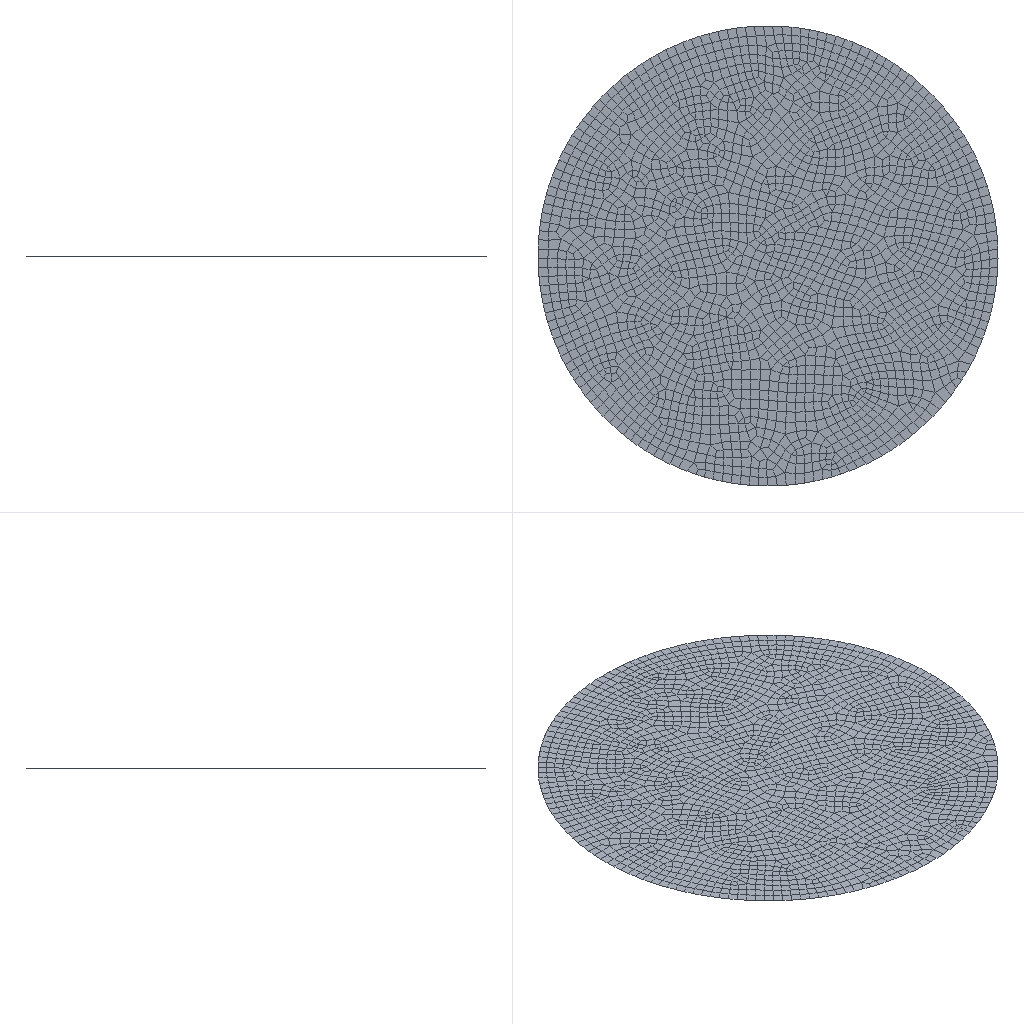Simulation study | abaqus
Set-up summary:
category,name,step,type,value,unit,region
solver,abaqus
solver,version,,,Abaqus/Explicit 2020
units,not stated in the deck,,not stated
analysis,deck,,transient,transient
load_step,Step-1,Step-1,transient,nlgeom=True
contact,interactions,,,general=1 pairs=0 ties=0
load_step,requested,,,1
mesh,nodes,,,8330
mesh,elements,,,8334
element_type,S3,,shell,63
element_type,S4R,,shell,2322
element_type,R3D3,,rigid,114
element_type,R3D4,,rigid,5835
load,load commands in deck,,count,1
bc,support commands in deck,,count,1
material,MATERIAL-1,,in results
check,setup vs results,,match,"per instance, exact: element labels, types and connectivity; labels of the nodes the elements use; coordinates of those nodes at SINGLE_PRECISION in 2 of 2 instance(s)"
Abaqus input file, long lists of numbers shortened:
*Heading
** Job name: Job-chongya Model name: Model-1
** Generated by: Abaqus/CAE 2020
*Preprint, echo=NO, model=NO, history=NO, contact=NO
**
** PARTS
**
*Part, name=p
*Node
      1,   5.989,  -49.64,           0.
      2,   11.891,  -48.565,           0.
** (2431 more lines like these left out)
*Element, type=S3
 1,   92, 1222,  796
 2, 1139, 1038, 1102
** (61 more lines like these left out)
*Element, type=S4R
  64,  717,  744,  663,  615
  65, 2106,  807,  473,  666
** (2320 more lines like these left out)
*Nset, nset=Set-1, generate
    1,  2433,     1
*Elset, elset=Set-1, generate
    1,  2385,     1
** Section: Section-1
*Shell Section, elset=Set-1, material=Material-1
1., 5
*End Part
**
*Part, name=work
*Node
      1,  -17.,  -19.639,   54.814
      2,  -17.,  -19.639,          56.
** (5894 more lines like these left out)
*Element, type=R3D4
 1,   1,  93, 156,   2
 2,  93,  94, 157, 156
** (5833 more lines like these left out)
*Element, type=R3D3
3034, 3552, 3563, 3559
3035, 3613, 3607, 3612
** (112 more lines like these left out)
*Node
   5897,  -5.65,  -26.539,          85.
*Nset, nset=work-RefPt_, internal
5897,
*Elset, elset=work, generate
    1,  5949,     1
*End Part
**
**
** ASSEMBLY
**
*Assembly, name=Assembly
**
*Instance, name=p-1, part=p
  -17.,     0.8613,    51.425
*End Instance
**
*Instance, name=work-1, part=work
*End Instance
**
*Nset, nset=Set-1, instance=work-1
 5897,
*Elset, elset=_Surf-1_SPOS, internal, instance=p-1, generate
    1,  2385,     1
*Surface, type=ELEMENT, name=Surf-1
_Surf-1_SPOS, SPOS
*Rigid Body, ref node=work-1.work-RefPt_, elset=work-1.work
*End Assembly
*Amplitude, name=Amp-1
             0.,              0.,            0.01,              1.
**
** MATERIALS
**
*Material, name=Material-1
*Density
 2.7e-09,
*Elastic
72000., 0.3
**
** INTERACTION PROPERTIES
**
*Surface Interaction, name=IntProp-1
*Friction
 0.3,
*Surface Behavior, pressure-overclosure=HARD
** ----------------------------------------------------------------
**
** STEP: Step-1
**
*Step, name=Step-1, nlgeom=YES
*Dynamic, Explicit
, 0.01
*Bulk Viscosity
0.06, 1.2
**
** BOUNDARY CONDITIONS
**
** Name: BC-1 Type: 对称/反对称/完全固定
*Boundary
Set-1, ENCASTRE
**
** LOADS
**
** Name: Load-1   Type: Pressure
*Dsload, amplitude=Amp-1
Surf-1, P, -20.
**
** INTERACTIONS
**
** Interaction: Int-1
*Contact, op=NEW
*Contact Inclusions, ALL EXTERIOR
*Contact Property Assignment
 ,  , IntProp-1
**
** OUTPUT REQUESTS
**
*Restart, write, number interval=1, time marks=NO
**
** FIELD OUTPUT: F-Output-1
**
*Output, field
*Node Output
A, RF, U, V
*Element Output, directions=YES
E, EVF, LE, MISES, MISESMAX, MISESONLY, PE, PEEQ, PEEQVAVG, PEVAVG, PRESSONLY, S, SEQUT, SSAVG, SVAVG, YIELDPOT
*Contact Output
CSTRESS,
**
** HISTORY OUTPUT: H-Output-1
**
*Output, history, variable=PRESELECT
*End Step
Results summary:
result,step,Step-1,completed,increments=80491 time=0.01/0.01
result,analysis,,,transient
result,last_loadstep,,,1
result,analysis steps,,count,1
result,primary field,,,"U, UR"
result,reaction total,,FX,-53.241,model units
result,reaction total,,FY,-233.998,model units
result,reaction total,,FZ,-80410.32,model units